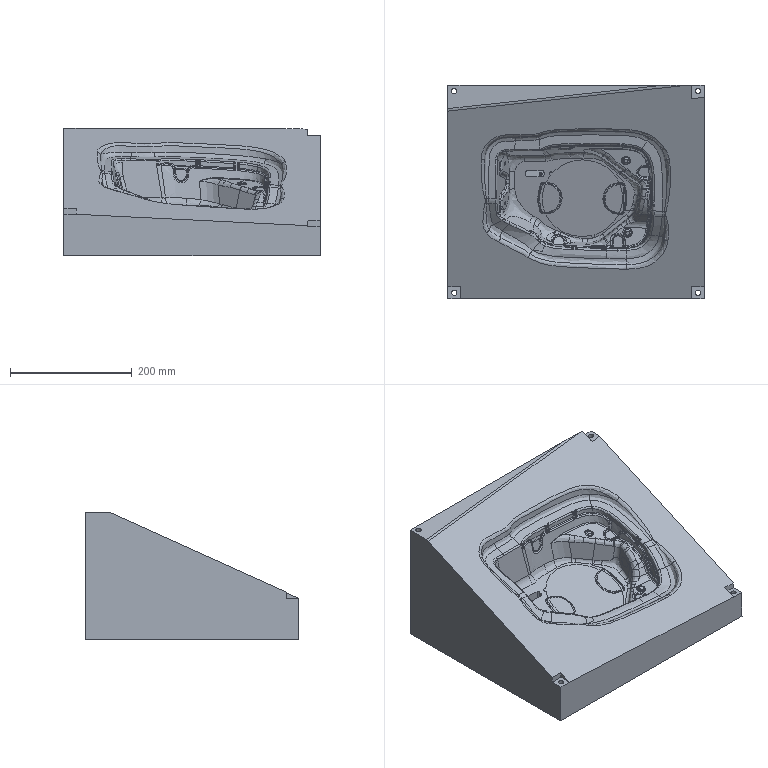CAM job | NX | 3-axis milling | part box 420 x 350 x 208.3 mm | stock box 420 x 350 x 208.3 mm
Tools:
number,name,description,diameter,corner_radius,flute_length,length,flutes
0,D40R5,Milling Tool-5 Parameters,40.0,5.0,50.0,75.0,2
0,D16R0.8,Milling Tool-5 Parameters,16.0,0.8,50.0,75.0,2
0,B10,Milling Tool-Ball Mill,10.0,5.0,50.0,75.0,2
Operations:
program,operation,operation_type,tool,method,geometry_group,spindle_rpm,surface_speed,feed_per_tooth,feed_cut,feed_plunge,cut_length_mm,path_length_mm,cut_time_min,machine_time_min
A01,CAVITY_MILL,CavityMilling,D40R5,METHOD,WORKPIECE,1400.0,175.0,0.9286,2600.0,100.0,790664.111,802994.912,304.102,305.335
A01,CAVITY_MILL_COPY,CavityMilling,D16R0.8,METHOD,WORKPIECE,1900.0,95.0,0.7895,3000.0,100.0,218041.655,220587.633,72.681,72.935
A01,CAVITY_MILL_COPY_COPY,CavityMilling,B10,METHOD,WORKPIECE,1900.0,95.0,0.7895,3000.0,100.0,39055.146,62678.239,13.018,15.381